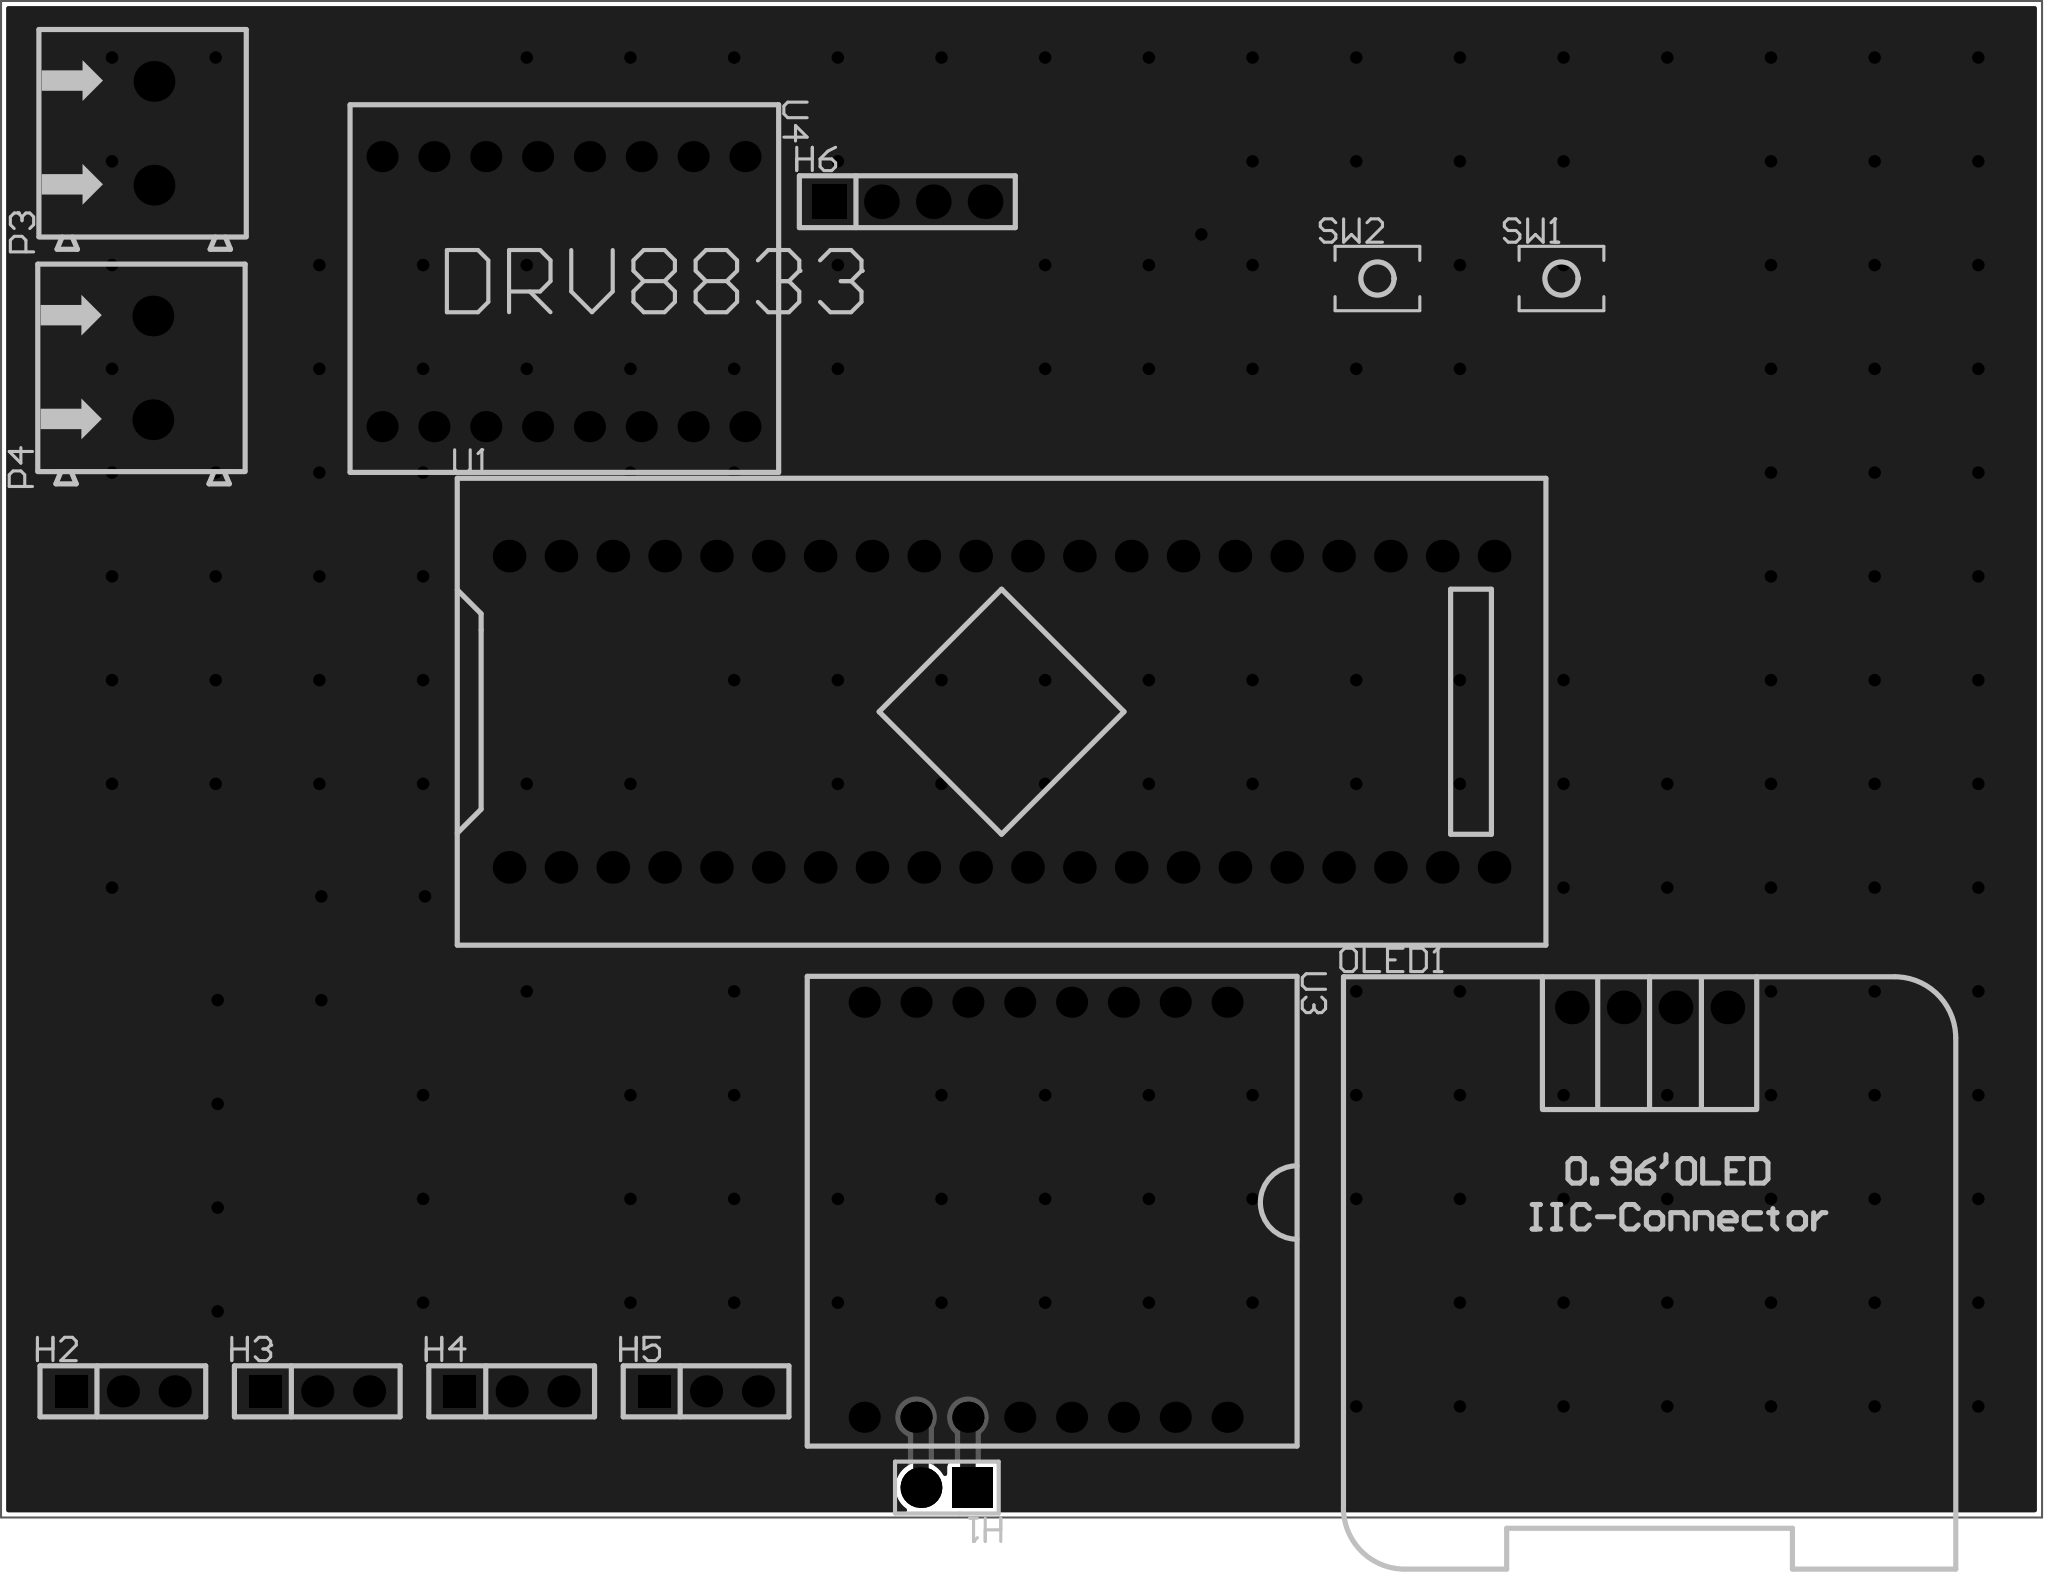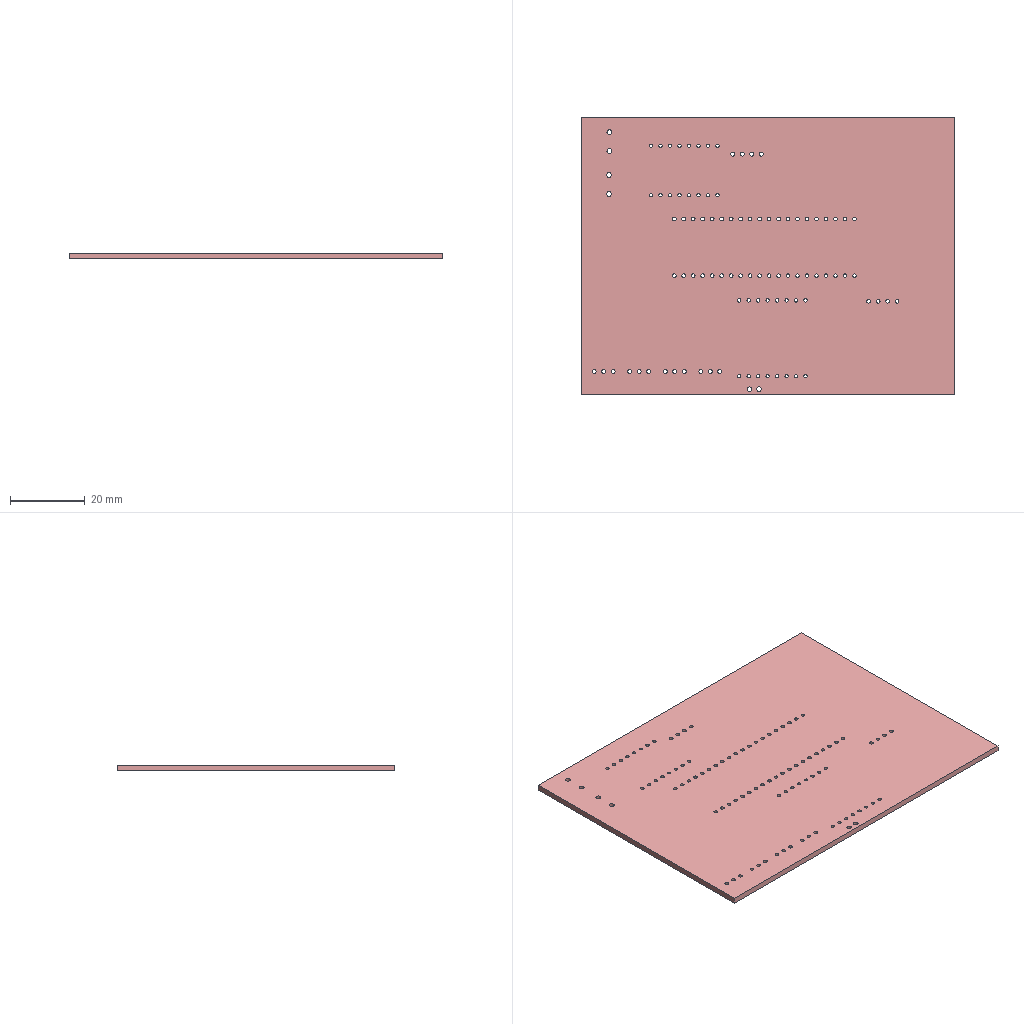Circuit board layout | Altium Designer | box 100 x 74.2 x 1.6 mm
Layer stack:
# Altium Designer layer stack of  (unit mm; dielectric type: 0 none, 1 core, 2 prepreg, 3 surface material)
index,name,kind,layer,copper_thickness_mm,dielectric_type,dielectric_thickness_mm,dielectric_material,dielectric_constant
0,Top Paste Mask Layer,other,,,,,,
1,Top Silkscreen Layer,other,,,,,,
2,Top Solder Mask Layer,dielectric,,,3,0.01,,3.3
3,Top Layer,copper,Top Layer,0.035,,,,
4,Dielectric1,dielectric,,,3,1.51,FR4,4.5
5,Bottom Layer,copper,Bottom Layer,0.035,,,,
6,Bottom Solder Mask Layer,dielectric,,,3,0.01,,3.3
7,Bottom Silkscreen Layer,other,,,,,,
8,Bottom Paste Mask Layer,other,,,,,,
# drill layer pairs: low layer,high layer
drill_pair,Top Layer,Bottom Layer
Part placement:
Designator,Comment,Layer,Footprint,Center-X(mm),Center-Y(mm),Rotation
H1,HX PH254-01-02-Z-L11.5 male header connector,TopLayer,HDR-TH_2P-P2.54-V-M,128.129,80.634,180
OLED1,,TopLayer,0.96OLED_4P,162.56,104.14,0
SW1,,TopLayer,Key_SMD_3x4x2,158.242,139.827,0
SW2,,TopLayer,Key_SMD_3x4x2,149.225,139.827,0
U1,STM32F103C8T6,TopLayer,CONN-TH_L53.3-W22.9_STM32F103C8T6-CARD,130.81,118.618,0
P3,WJ500V-5.08-2P,TopLayer,CONN-TH_2P-P5.00_WJ500V-5.08-2P,89.281,146.939,90
P4,WJ500V-5.08-2P,TopLayer,CONN-TH_2P-P5.00_WJ500V-5.08-2P,89.225,135.453,90
U4,,TopLayer,DRV8833,109.347,139.186,270
U3,,TopLayer,MY2490-16P,132.969,94.234,270
H2,,TopLayer,HDR-TH_3P-P2.54-V-F,87.757,85.344,0
H3,,TopLayer,HDR-TH_3P-P2.54-V-F,97.282,85.344,0
H4,,TopLayer,HDR-TH_3P-P2.54-V-F,106.807,85.344,0
H5,,TopLayer,HDR-TH_3P-P2.54-V-F,116.332,85.344,0
H6,,TopLayer,HDR-TH_4P-P2.54-V-F,126.192,143.588,0
Pad and via stacks:
# Altium Designer via and pad stacks of  (unit mm). Each distinct definition once, with the count of objects using it.
# via: kind,start_layer,end_layer,hole_mm,diameter_mm,mode(0 simple;1 top-mid-bottom;2 full stack),diameter_per_layer,count,example_net
# pad: kind,layer,hole_mm,hole_type(0 round;1 square;2 slot),plating,top_size,top_shape(1 round;2 rect;3 octagon;9 rounded rect),mid_size,bottom_size,mode,footprint,size_per_layer,count,example
pad,Multi-Layer,1.2,0,plated,2x2,2,2x2,2x2,0,HDR-TH_2P-P2.54-V-M,,1,H1.1
pad,Multi-Layer,1.2,0,plated,2x2,1,2x2,2x2,0,HDR-TH_2P-P2.54-V-M,,1,H1.2
pad,Multi-Layer,1,0,plated,1.65x1.65,1,1.65x1.65,1.65x1.65,0,0.96OLED_4P,,4,OLED1.4
pad,Multi-Layer,1,0,plated,1.6x1.6,1,1.6x1.6,1.6x1.6,0,CONN-TH_L53.3-W22.9_STM32F103C8T6-CARD,,40,U1.1
pad,Multi-Layer,1.3,0,plated,2x2,1,2x2,2x2,0,CONN-TH_2P-P5.00_WJ500V-5.08-2P,,4,P3.2
pad,Multi-Layer,0.9144,0,plated,1.524x1.524,1,1.524x1.524,1.524x1.524,0,DRV8833,,16,U4.1
pad,Multi-Layer,0.9144,0,plated,1.524x1.524,1,1.524x1.524,1.524x1.524,0,MY2490-16P,,16,U3.1
pad,Multi-Layer,1.02,0,plated,1.575x1.575,1,1.575x1.575,1.575x1.575,0,HDR-TH_3P-P2.54-V-F,,8,H2.3
pad,Multi-Layer,1.02,0,plated,1.575x1.575,2,1.575x1.575,1.575x1.575,0,HDR-TH_3P-P2.54-V-F,,4,H2.1
pad,Multi-Layer,1.1,0,plated,1.7x1.7,2,1.7x1.7,1.7x1.7,0,HDR-TH_4P-P2.54-V-F,,1,H6.1
pad,Multi-Layer,1.1,0,plated,1.7x1.7,1,1.7x1.7,1.7x1.7,0,HDR-TH_4P-P2.54-V-F,,3,H6.2
pad,Top Layer,0,0,plated,1.53x1.36,2,1.53x1.36,1.53x1.36,0,Key_SMD_3x4x2,,4,SW1.1
via,Top Layer,Bottom Layer,0.3048,0.61,0,,175,GND
Copper pours:
name,layer,net,type(0 solid;1 hatched;2 none)
Top Layer-GND,Top Layer,GND,0
Bottom Layer-GND,Bottom Layer,GND,0